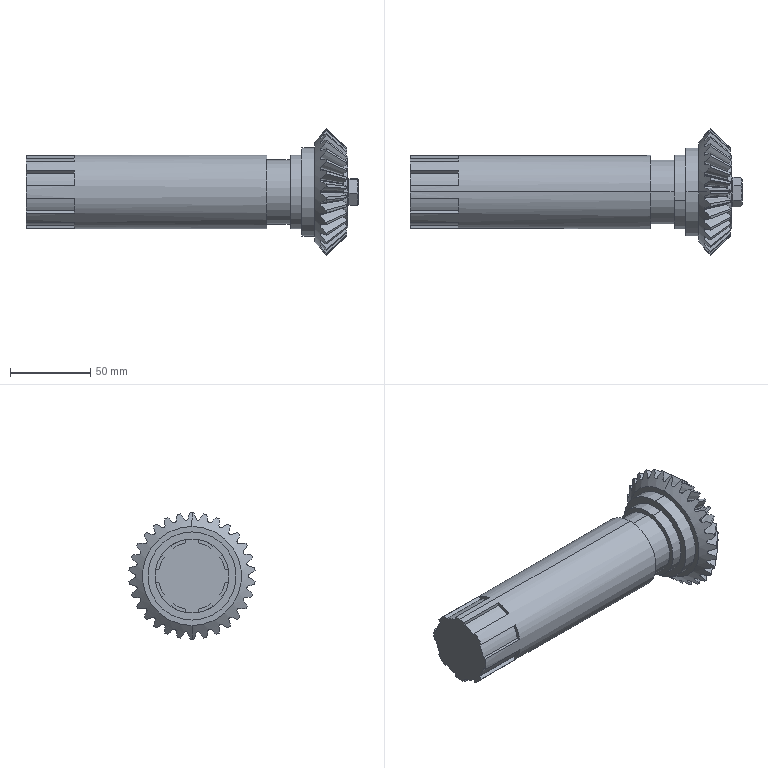Part | SolidWorks | 6 solids | 376 faces | box 206.989 x 78.579 x 78.841 mm | volume 358378 mm3 | cone 148 | spline 90 | cylinder 70 | plane 60 | torus 8 | commonest cylinder face diameters 10 x32 42.078 x8 12 x5 39 x5 1.2 x4 40 x4